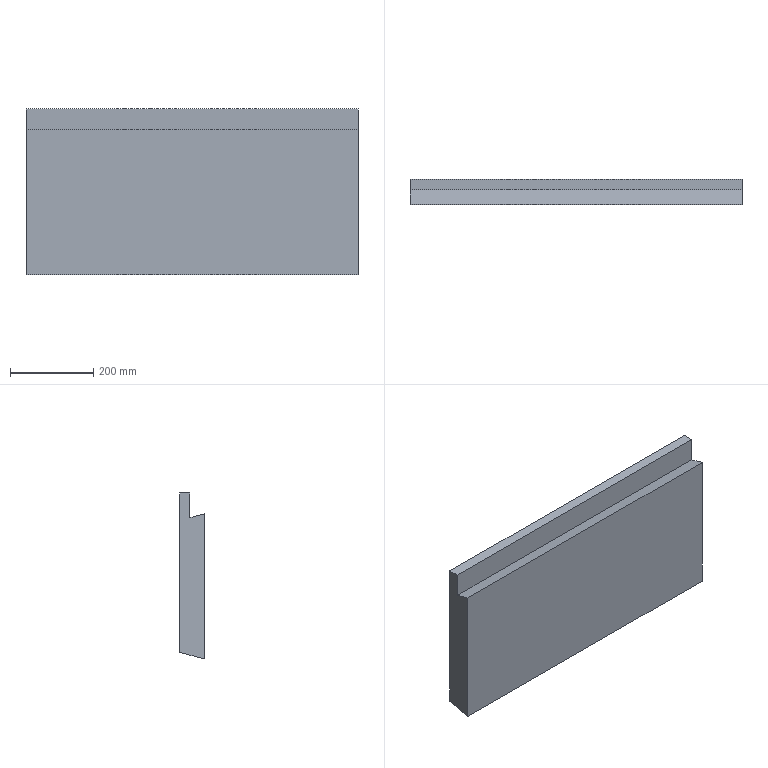Part | SolidWorks | features Extrusion 1 | 1 solid | 8 faces | box 800 x 60 x 400 mm | volume 17282858 mm3 | plane 8
STEP:
#1=CARTESIAN_POINT('',(-400.,0.,0.));
#2=VERTEX_POINT('',#1);
#3=CARTESIAN_POINT('',(-400.,0.,-350.));
#4=VERTEX_POINT('',#3);
#5=CARTESIAN_POINT('',(-400.,0.,0.));
#6=DIRECTION('',(0.,0.,-1.));
#7=VECTOR('',#6,1000.);
#8=LINE('',#5,#7);
#9=EDGE_CURVE('',#2,#4,#8,.T.);
#10=ORIENTED_EDGE('',*,*,#9,.T.);
#11=CARTESIAN_POINT('',(400.,0.,-350.));
#12=VERTEX_POINT('',#11);
#13=CARTESIAN_POINT('',(400.,0.,-350.));
#14=DIRECTION('',(-1.,0.,0.));
#15=VECTOR('',#14,1000.);
#16=LINE('',#13,#15);
#17=EDGE_CURVE('',#12,#4,#16,.T.);
#18=ORIENTED_EDGE('',*,*,#17,.F.);
#19=CARTESIAN_POINT('',(400.,0.,0.));
#20=VERTEX_POINT('',#19);
#21=CARTESIAN_POINT('',(400.,0.,0.));
#22=DIRECTION('',(0.,0.,-1.));
#23=VECTOR('',#22,1000.);
#24=LINE('',#21,#23);
#25=EDGE_CURVE('',#20,#12,#24,.T.);
#26=ORIENTED_EDGE('',*,*,#25,.F.);
#27=CARTESIAN_POINT('',(400.,0.,0.));
#28=DIRECTION('',(-1.,0.,0.));
#29=VECTOR('',#28,1000.);
#30=LINE('',#27,#29);
#31=EDGE_CURVE('',#20,#2,#30,.T.);
#32=ORIENTED_EDGE('',*,*,#31,.T.);
#33=EDGE_LOOP('',(#10,#18,#26,#32));
#34=FACE_OUTER_BOUND('',#33,.T.);
#35=CARTESIAN_POINT('',(400.,0.,0.));
#36=DIRECTION('',(0.,1.,0.));
#37=DIRECTION('',(0.,0.,1.));
#38=AXIS2_PLACEMENT_3D('',#35,#36,#37);
#39=PLANE('',#38);
#40=ADVANCED_FACE('',(#34),#39,.F.);
#41=CARTESIAN_POINT('',(-400.,60.,-333.923));
#42=VERTEX_POINT('',#41);
#43=CARTESIAN_POINT('',(-400.,0.,-350.));
#44=DIRECTION('',(0.,0.9659,0.2588));
#45=VECTOR('',#44,1000.);
#46=LINE('',#43,#45);
#47=EDGE_CURVE('',#4,#42,#46,.T.);
#48=ORIENTED_EDGE('',*,*,#47,.T.);
#49=CARTESIAN_POINT('',(400.,60.,-333.923));
#50=VERTEX_POINT('',#49);
#51=CARTESIAN_POINT('',(400.,60.,-333.923));
#52=DIRECTION('',(-1.,0.,0.));
#53=VECTOR('',#52,1000.);
#54=LINE('',#51,#53);
#55=EDGE_CURVE('',#50,#42,#54,.T.);
#56=ORIENTED_EDGE('',*,*,#55,.F.);
#57=CARTESIAN_POINT('',(400.,0.,-350.));
#58=DIRECTION('',(0.,0.9659,0.2588));
#59=VECTOR('',#58,1000.);
#60=LINE('',#57,#59);
#61=EDGE_CURVE('',#12,#50,#60,.T.);
#62=ORIENTED_EDGE('',*,*,#61,.F.);
#63=ORIENTED_EDGE('',*,*,#17,.T.);
#64=EDGE_LOOP('',(#48,#56,#62,#63));
#65=FACE_OUTER_BOUND('',#64,.T.);
#66=CARTESIAN_POINT('',(400.,0.,-350.));
#67=DIRECTION('',(0.,-0.2588,0.9659));
#68=DIRECTION('',(0.,-0.9659,-0.2588));
#69=AXIS2_PLACEMENT_3D('',#66,#67,#68);
#70=PLANE('',#69);
#71=ADVANCED_FACE('',(#65),#70,.F.);
#72=CARTESIAN_POINT('',(-400.,60.,50.));
#73=VERTEX_POINT('',#72);
#74=CARTESIAN_POINT('',(-400.,60.,-333.923));
#75=DIRECTION('',(0.,0.,1.));
#76=VECTOR('',#75,1000.);
#77=LINE('',#74,#76);
#78=EDGE_CURVE('',#42,#73,#77,.T.);
#79=ORIENTED_EDGE('',*,*,#78,.T.);
#80=CARTESIAN_POINT('',(400.,60.,50.));
#81=VERTEX_POINT('',#80);
#82=CARTESIAN_POINT('',(400.,60.,50.));
#83=DIRECTION('',(-1.,0.,0.));
#84=VECTOR('',#83,1000.);
#85=LINE('',#82,#84);
#86=EDGE_CURVE('',#81,#73,#85,.T.);
#87=ORIENTED_EDGE('',*,*,#86,.F.);
#88=CARTESIAN_POINT('',(400.,60.,-333.923));
#89=DIRECTION('',(0.,0.,1.));
#90=VECTOR('',#89,1000.);
#91=LINE('',#88,#90);
#92=EDGE_CURVE('',#50,#81,#91,.T.);
#93=ORIENTED_EDGE('',*,*,#92,.F.);
#94=ORIENTED_EDGE('',*,*,#55,.T.);
#95=EDGE_LOOP('',(#79,#87,#93,#94));
#96=FACE_OUTER_BOUND('',#95,.T.);
#97=CARTESIAN_POINT('',(400.,60.,-333.923));
#98=DIRECTION('',(0.,-1.,0.));
#99=DIRECTION('',(0.,0.,-1.));
#100=AXIS2_PLACEMENT_3D('',#97,#98,#99);
#101=PLANE('',#100);
#102=ADVANCED_FACE('',(#96),#101,.F.);
#103=CARTESIAN_POINT('',(-400.,35.,50.));
#104=VERTEX_POINT('',#103);
#105=CARTESIAN_POINT('',(-400.,60.,50.));
#106=DIRECTION('',(0.,-1.,0.));
#107=VECTOR('',#106,1000.);
#108=LINE('',#105,#107);
#109=EDGE_CURVE('',#73,#104,#108,.T.);
#110=ORIENTED_EDGE('',*,*,#109,.T.);
#111=CARTESIAN_POINT('',(400.,35.,50.));
#112=VERTEX_POINT('',#111);
#113=CARTESIAN_POINT('',(400.,35.,50.));
#114=DIRECTION('',(-1.,0.,0.));
#115=VECTOR('',#114,1000.);
#116=LINE('',#113,#115);
#117=EDGE_CURVE('',#112,#104,#116,.T.);
#118=ORIENTED_EDGE('',*,*,#117,.F.);
#119=CARTESIAN_POINT('',(400.,60.,50.));
#120=DIRECTION('',(0.,-1.,0.));
#121=VECTOR('',#120,1000.);
#122=LINE('',#119,#121);
#123=EDGE_CURVE('',#81,#112,#122,.T.);
#124=ORIENTED_EDGE('',*,*,#123,.F.);
#125=ORIENTED_EDGE('',*,*,#86,.T.);
#126=EDGE_LOOP('',(#110,#118,#124,#125));
#127=FACE_OUTER_BOUND('',#126,.T.);
#128=CARTESIAN_POINT('',(400.,60.,50.));
#129=DIRECTION('',(0.,0.,-1.));
#130=DIRECTION('',(0.,1.,0.));
#131=AXIS2_PLACEMENT_3D('',#128,#129,#130);
#132=PLANE('',#131);
#133=ADVANCED_FACE('',(#127),#132,.F.);
#134=CARTESIAN_POINT('',(-400.,35.,-9.378));
#135=VERTEX_POINT('',#134);
#136=CARTESIAN_POINT('',(-400.,35.,50.));
#137=DIRECTION('',(0.,0.,-1.));
#138=VECTOR('',#137,1000.);
#139=LINE('',#136,#138);
#140=EDGE_CURVE('',#104,#135,#139,.T.);
#141=ORIENTED_EDGE('',*,*,#140,.T.);
#142=CARTESIAN_POINT('',(400.,35.,-9.378));
#143=VERTEX_POINT('',#142);
#144=CARTESIAN_POINT('',(400.,35.,-9.378));
#145=DIRECTION('',(-1.,0.,0.));
#146=VECTOR('',#145,1000.);
#147=LINE('',#144,#146);
#148=EDGE_CURVE('',#143,#135,#147,.T.);
#149=ORIENTED_EDGE('',*,*,#148,.F.);
#150=CARTESIAN_POINT('',(400.,35.,50.));
#151=DIRECTION('',(0.,0.,-1.));
#152=VECTOR('',#151,1000.);
#153=LINE('',#150,#152);
#154=EDGE_CURVE('',#112,#143,#153,.T.);
#155=ORIENTED_EDGE('',*,*,#154,.F.);
#156=ORIENTED_EDGE('',*,*,#117,.T.);
#157=EDGE_LOOP('',(#141,#149,#155,#156));
#158=FACE_OUTER_BOUND('',#157,.T.);
#159=CARTESIAN_POINT('',(400.,35.,50.));
#160=DIRECTION('',(0.,1.,0.));
#161=DIRECTION('',(0.,0.,1.));
#162=AXIS2_PLACEMENT_3D('',#159,#160,#161);
#163=PLANE('',#162);
#164=ADVANCED_FACE('',(#158),#163,.F.);
#165=CARTESIAN_POINT('',(-400.,35.,-9.378));
#166=DIRECTION('',(0.,-0.9659,0.2588));
#167=VECTOR('',#166,1000.);
#168=LINE('',#165,#167);
#169=EDGE_CURVE('',#135,#2,#168,.T.);
#170=ORIENTED_EDGE('',*,*,#169,.T.);
#171=ORIENTED_EDGE('',*,*,#31,.F.);
#172=CARTESIAN_POINT('',(400.,35.,-9.378));
#173=DIRECTION('',(0.,-0.9659,0.2588));
#174=VECTOR('',#173,1000.);
#175=LINE('',#172,#174);
#176=EDGE_CURVE('',#143,#20,#175,.T.);
#177=ORIENTED_EDGE('',*,*,#176,.F.);
#178=ORIENTED_EDGE('',*,*,#148,.T.);
#179=EDGE_LOOP('',(#170,#171,#177,#178));
#180=FACE_OUTER_BOUND('',#179,.T.);
#181=CARTESIAN_POINT('',(400.,35.,-9.378));
#182=DIRECTION('',(0.,-0.2588,-0.9659));
#183=DIRECTION('',(0.,0.9659,-0.2588));
#184=AXIS2_PLACEMENT_3D('',#181,#182,#183);
#185=PLANE('',#184);
#186=ADVANCED_FACE('',(#180),#185,.F.);
#187=ORIENTED_EDGE('',*,*,#25,.T.);
#188=ORIENTED_EDGE('',*,*,#61,.T.);
#189=ORIENTED_EDGE('',*,*,#92,.T.);
#190=ORIENTED_EDGE('',*,*,#123,.T.);
#191=ORIENTED_EDGE('',*,*,#154,.T.);
#192=ORIENTED_EDGE('',*,*,#176,.T.);
#193=EDGE_LOOP('',(#187,#188,#189,#190,#191,#192));
#194=FACE_OUTER_BOUND('',#193,.T.);
#195=CARTESIAN_POINT('',(400.,0.,0.));
#196=DIRECTION('',(-1.,0.,0.));
#197=DIRECTION('',(0.,0.,1.));
#198=AXIS2_PLACEMENT_3D('',#195,#196,#197);
#199=PLANE('',#198);
#200=ADVANCED_FACE('',(#194),#199,.F.);
#201=ORIENTED_EDGE('',*,*,#9,.F.);
#202=ORIENTED_EDGE('',*,*,#169,.F.);
#203=ORIENTED_EDGE('',*,*,#140,.F.);
#204=ORIENTED_EDGE('',*,*,#109,.F.);
#205=ORIENTED_EDGE('',*,*,#78,.F.);
#206=ORIENTED_EDGE('',*,*,#47,.F.);
#207=EDGE_LOOP('',(#201,#202,#203,#204,#205,#206));
#208=FACE_OUTER_BOUND('',#207,.T.);
#209=CARTESIAN_POINT('',(-400.,0.,0.));
#210=DIRECTION('',(-1.,0.,0.));
#211=DIRECTION('',(0.,0.,1.));
#212=AXIS2_PLACEMENT_3D('',#209,#210,#211);
#213=PLANE('',#212);
#214=ADVANCED_FACE('',(#208),#213,.T.);
#215=CLOSED_SHELL('',(#40,#71,#102,#133,#164,#186,#200,#214));
#216=MANIFOLD_SOLID_BREP('',#215);
#217=CARTESIAN_POINT('',(0.,0.,0.));
#218=DIRECTION('',(0.,0.,1.));
#219=DIRECTION('',(1.,0.,0.));
#220=AXIS2_PLACEMENT_3D('',#217,#218,#219);
#221=(LENGTH_UNIT()NAMED_UNIT(*)SI_UNIT(.MILLI.,.METRE.));
#222=UNCERTAINTY_MEASURE_WITH_UNIT(LENGTH_MEASURE(0.00001),#221,'','');
#223=(NAMED_UNIT(*)PLANE_ANGLE_UNIT()SI_UNIT($,.RADIAN.));
#224=(NAMED_UNIT(*)SI_UNIT($,.STERADIAN.)SOLID_ANGLE_UNIT());
#225=(GEOMETRIC_REPRESENTATION_CONTEXT(3)GLOBAL_UNCERTAINTY_ASSIGNED_CONTEXT((#222))GLOBAL_UNIT_ASSIGNED_CONTEXT((#221,#223,#224))REPRESENTATION_CONTEXT('',''));
#226=ADVANCED_BREP_SHAPE_REPRESENTATION('',(#216,#220),#225);